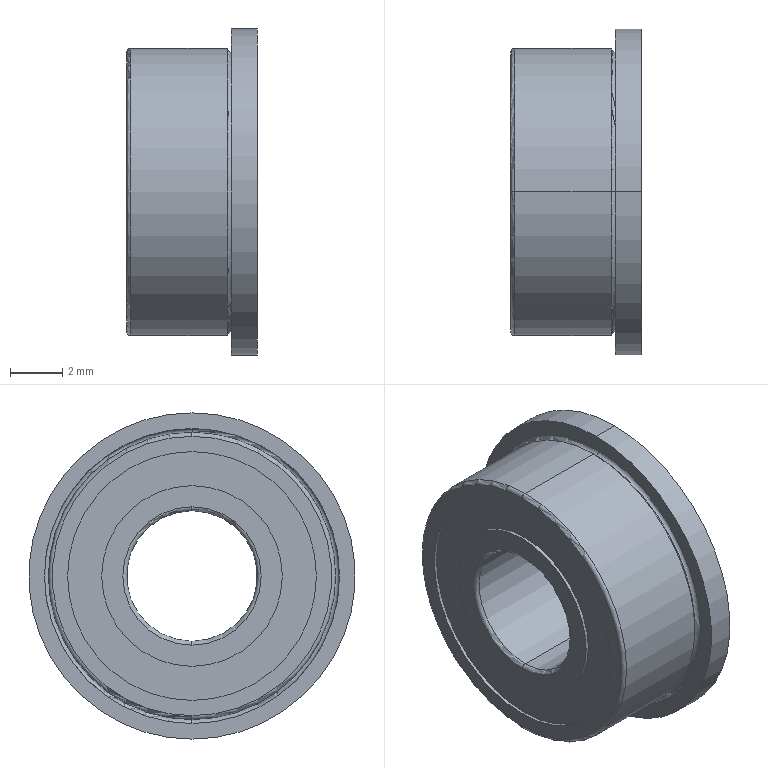Part | SolidWorks | features RefAxis 3, 3DProfileFeature 1, Revolution 1 | 1 solid | 31 faces | box 5 x 12.5 x 12.5 mm | volume 394.425 mm3 | cylinder 14 | torus 10 | plane 7 | commonest cylinder face diameters 6.92 x4 9.534 x4 5 x2 11 x2 12.5 x2
STEP:
#1=CARTESIAN_POINT('',(3.85,0.,5.5));
#2=VERTEX_POINT('',#1);
#3=CARTESIAN_POINT('',(4.,0.,5.35));
#4=VERTEX_POINT('',#3);
#5=CARTESIAN_POINT('',(4.,0.,5.5));
#6=DIRECTION('',(0.,-1.,0.));
#7=DIRECTION('',(0.,0.,-1.));
#8=AXIS2_PLACEMENT_3D('',#5,#6,#7);
#9=CIRCLE('',#8,0.15);
#10=EDGE_CURVE('',#2,#4,#9,.T.);
#11=ORIENTED_EDGE('',*,*,#10,.T.);
#12=CARTESIAN_POINT('',(4.,0.,-5.35));
#13=VERTEX_POINT('',#12);
#14=CARTESIAN_POINT('',(4.,0.,0.));
#15=DIRECTION('',(-1.,0.,0.));
#16=DIRECTION('',(0.,0.,1.));
#17=AXIS2_PLACEMENT_3D('',#14,#15,#16);
#18=CIRCLE('',#17,5.35);
#19=EDGE_CURVE('',#4,#13,#18,.T.);
#20=ORIENTED_EDGE('',*,*,#19,.T.);
#21=CARTESIAN_POINT('',(3.85,0.,-5.5));
#22=VERTEX_POINT('',#21);
#23=CARTESIAN_POINT('',(4.,0.,-5.5));
#24=DIRECTION('',(0.,1.,0.));
#25=DIRECTION('',(0.,0.,1.));
#26=AXIS2_PLACEMENT_3D('',#23,#24,#25);
#27=CIRCLE('',#26,0.15);
#28=EDGE_CURVE('',#22,#13,#27,.T.);
#29=ORIENTED_EDGE('',*,*,#28,.F.);
#30=CARTESIAN_POINT('',(3.85,0.,0.));
#31=DIRECTION('',(-1.,0.,0.));
#32=DIRECTION('',(0.,0.,1.));
#33=AXIS2_PLACEMENT_3D('',#30,#31,#32);
#34=CIRCLE('',#33,5.5);
#35=EDGE_CURVE('',#2,#22,#34,.T.);
#36=ORIENTED_EDGE('',*,*,#35,.F.);
#37=EDGE_LOOP('',(#11,#20,#29,#36));
#38=FACE_OUTER_BOUND('',#37,.T.);
#39=CARTESIAN_POINT('',(4.,0.,0.));
#40=DIRECTION('',(-1.,0.,0.));
#41=DIRECTION('',(0.,0.,1.));
#42=AXIS2_PLACEMENT_3D('',#39,#40,#41);
#43=TOROIDAL_SURFACE('',#42,5.5,0.15);
#44=ADVANCED_FACE('',(#38),#43,.F.);
#45=ORIENTED_EDGE('',*,*,#28,.T.);
#46=CARTESIAN_POINT('',(4.,0.,0.));
#47=DIRECTION('',(-1.,0.,0.));
#48=DIRECTION('',(0.,0.,1.));
#49=AXIS2_PLACEMENT_3D('',#46,#47,#48);
#50=CIRCLE('',#49,5.35);
#51=EDGE_CURVE('',#13,#4,#50,.T.);
#52=ORIENTED_EDGE('',*,*,#51,.T.);
#53=ORIENTED_EDGE('',*,*,#10,.F.);
#54=CARTESIAN_POINT('',(3.85,0.,0.));
#55=DIRECTION('',(-1.,0.,0.));
#56=DIRECTION('',(0.,0.,1.));
#57=AXIS2_PLACEMENT_3D('',#54,#55,#56);
#58=CIRCLE('',#57,5.5);
#59=EDGE_CURVE('',#22,#2,#58,.T.);
#60=ORIENTED_EDGE('',*,*,#59,.F.);
#61=EDGE_LOOP('',(#45,#52,#53,#60));
#62=FACE_OUTER_BOUND('',#61,.T.);
#63=CARTESIAN_POINT('',(4.,0.,0.));
#64=DIRECTION('',(-1.,0.,0.));
#65=DIRECTION('',(0.,0.,1.));
#66=AXIS2_PLACEMENT_3D('',#63,#64,#65);
#67=TOROIDAL_SURFACE('',#66,5.5,0.15);
#68=ADVANCED_FACE('',(#62),#67,.F.);
#69=ORIENTED_EDGE('',*,*,#35,.T.);
#70=CARTESIAN_POINT('',(0.15,0.,-5.5));
#71=VERTEX_POINT('',#70);
#72=CARTESIAN_POINT('',(11.,0.,-5.5));
#73=DIRECTION('',(-1.,0.,0.));
#74=VECTOR('',#73,1000.);
#75=LINE('',#72,#74);
#76=EDGE_CURVE('',#22,#71,#75,.T.);
#77=ORIENTED_EDGE('',*,*,#76,.T.);
#78=CARTESIAN_POINT('',(0.15,0.,5.5));
#79=VERTEX_POINT('',#78);
#80=CARTESIAN_POINT('',(0.15,0.,0.));
#81=DIRECTION('',(-1.,0.,0.));
#82=DIRECTION('',(0.,0.,1.));
#83=AXIS2_PLACEMENT_3D('',#80,#81,#82);
#84=CIRCLE('',#83,5.5);
#85=EDGE_CURVE('',#79,#71,#84,.T.);
#86=ORIENTED_EDGE('',*,*,#85,.F.);
#87=CARTESIAN_POINT('',(11.,0.,5.5));
#88=DIRECTION('',(-1.,0.,0.));
#89=VECTOR('',#88,1000.);
#90=LINE('',#87,#89);
#91=EDGE_CURVE('',#2,#79,#90,.T.);
#92=ORIENTED_EDGE('',*,*,#91,.F.);
#93=EDGE_LOOP('',(#69,#77,#86,#92));
#94=FACE_OUTER_BOUND('',#93,.T.);
#95=CARTESIAN_POINT('',(11.,0.,0.));
#96=DIRECTION('',(-1.,0.,0.));
#97=DIRECTION('',(0.,0.,1.));
#98=AXIS2_PLACEMENT_3D('',#95,#96,#97);
#99=CYLINDRICAL_SURFACE('',#98,5.5);
#100=ADVANCED_FACE('',(#94),#99,.T.);
#101=ORIENTED_EDGE('',*,*,#51,.F.);
#102=CARTESIAN_POINT('',(4.,0.,-5.65));
#103=VERTEX_POINT('',#102);
#104=CARTESIAN_POINT('',(4.,0.,-5.5));
#105=DIRECTION('',(0.,1.,0.));
#106=DIRECTION('',(0.,0.,1.));
#107=AXIS2_PLACEMENT_3D('',#104,#105,#106);
#108=CIRCLE('',#107,0.15);
#109=EDGE_CURVE('',#13,#103,#108,.T.);
#110=ORIENTED_EDGE('',*,*,#109,.T.);
#111=CARTESIAN_POINT('',(4.,0.,5.65));
#112=VERTEX_POINT('',#111);
#113=CARTESIAN_POINT('',(4.,0.,0.));
#114=DIRECTION('',(-1.,0.,0.));
#115=DIRECTION('',(0.,0.,1.));
#116=AXIS2_PLACEMENT_3D('',#113,#114,#115);
#117=CIRCLE('',#116,5.65);
#118=EDGE_CURVE('',#103,#112,#117,.T.);
#119=ORIENTED_EDGE('',*,*,#118,.T.);
#120=CARTESIAN_POINT('',(4.,0.,5.5));
#121=DIRECTION('',(0.,-1.,0.));
#122=DIRECTION('',(0.,0.,-1.));
#123=AXIS2_PLACEMENT_3D('',#120,#121,#122);
#124=CIRCLE('',#123,0.15);
#125=EDGE_CURVE('',#4,#112,#124,.T.);
#126=ORIENTED_EDGE('',*,*,#125,.F.);
#127=EDGE_LOOP('',(#101,#110,#119,#126));
#128=FACE_OUTER_BOUND('',#127,.T.);
#129=CARTESIAN_POINT('',(4.,0.,0.));
#130=DIRECTION('',(-1.,0.,0.));
#131=DIRECTION('',(0.,0.,1.));
#132=AXIS2_PLACEMENT_3D('',#129,#130,#131);
#133=TOROIDAL_SURFACE('',#132,5.5,0.15);
#134=ADVANCED_FACE('',(#128),#133,.F.);
#135=CARTESIAN_POINT('',(5.,0.,6.25));
#136=VERTEX_POINT('',#135);
#137=CARTESIAN_POINT('',(5.,0.,-6.25));
#138=VERTEX_POINT('',#137);
#139=CARTESIAN_POINT('',(5.,0.,0.));
#140=DIRECTION('',(-1.,0.,0.));
#141=DIRECTION('',(0.,0.,1.));
#142=AXIS2_PLACEMENT_3D('',#139,#140,#141);
#143=CIRCLE('',#142,6.25);
#144=EDGE_CURVE('',#136,#138,#143,.T.);
#145=ORIENTED_EDGE('',*,*,#144,.T.);
#146=CARTESIAN_POINT('',(4.,0.,-6.25));
#147=VERTEX_POINT('',#146);
#148=CARTESIAN_POINT('',(11.,0.,-6.25));
#149=DIRECTION('',(-1.,0.,0.));
#150=VECTOR('',#149,1000.);
#151=LINE('',#148,#150);
#152=EDGE_CURVE('',#138,#147,#151,.T.);
#153=ORIENTED_EDGE('',*,*,#152,.T.);
#154=CARTESIAN_POINT('',(4.,0.,6.25));
#155=VERTEX_POINT('',#154);
#156=CARTESIAN_POINT('',(4.,0.,0.));
#157=DIRECTION('',(-1.,0.,0.));
#158=DIRECTION('',(0.,0.,1.));
#159=AXIS2_PLACEMENT_3D('',#156,#157,#158);
#160=CIRCLE('',#159,6.25);
#161=EDGE_CURVE('',#155,#147,#160,.T.);
#162=ORIENTED_EDGE('',*,*,#161,.F.);
#163=CARTESIAN_POINT('',(11.,0.,6.25));
#164=DIRECTION('',(-1.,0.,0.));
#165=VECTOR('',#164,1000.);
#166=LINE('',#163,#165);
#167=EDGE_CURVE('',#136,#155,#166,.T.);
#168=ORIENTED_EDGE('',*,*,#167,.F.);
#169=EDGE_LOOP('',(#145,#153,#162,#168));
#170=FACE_OUTER_BOUND('',#169,.T.);
#171=CARTESIAN_POINT('',(11.,0.,0.));
#172=DIRECTION('',(-1.,0.,0.));
#173=DIRECTION('',(0.,0.,1.));
#174=AXIS2_PLACEMENT_3D('',#171,#172,#173);
#175=CYLINDRICAL_SURFACE('',#174,6.25);
#176=ADVANCED_FACE('',(#170),#175,.T.);
#177=CARTESIAN_POINT('',(5.,0.,-4.767));
#178=VERTEX_POINT('',#177);
#179=CARTESIAN_POINT('',(5.,0.,4.767));
#180=VERTEX_POINT('',#179);
#181=CARTESIAN_POINT('',(5.,0.,0.));
#182=DIRECTION('',(-1.,0.,0.));
#183=DIRECTION('',(0.,0.,1.));
#184=AXIS2_PLACEMENT_3D('',#181,#182,#183);
#185=CIRCLE('',#184,4.767);
#186=EDGE_CURVE('',#178,#180,#185,.T.);
#187=ORIENTED_EDGE('',*,*,#186,.F.);
#188=CARTESIAN_POINT('',(4.88,0.,-4.767));
#189=VERTEX_POINT('',#188);
#190=CARTESIAN_POINT('',(11.,0.,-4.767));
#191=DIRECTION('',(-1.,0.,0.));
#192=VECTOR('',#191,1000.);
#193=LINE('',#190,#192);
#194=EDGE_CURVE('',#178,#189,#193,.T.);
#195=ORIENTED_EDGE('',*,*,#194,.T.);
#196=CARTESIAN_POINT('',(4.88,0.,4.767));
#197=VERTEX_POINT('',#196);
#198=CARTESIAN_POINT('',(4.88,0.,0.));
#199=DIRECTION('',(-1.,0.,0.));
#200=DIRECTION('',(0.,0.,1.));
#201=AXIS2_PLACEMENT_3D('',#198,#199,#200);
#202=CIRCLE('',#201,4.767);
#203=EDGE_CURVE('',#189,#197,#202,.T.);
#204=ORIENTED_EDGE('',*,*,#203,.T.);
#205=CARTESIAN_POINT('',(11.,0.,4.767));
#206=DIRECTION('',(-1.,0.,0.));
#207=VECTOR('',#206,1000.);
#208=LINE('',#205,#207);
#209=EDGE_CURVE('',#180,#197,#208,.T.);
#210=ORIENTED_EDGE('',*,*,#209,.F.);
#211=EDGE_LOOP('',(#187,#195,#204,#210));
#212=FACE_OUTER_BOUND('',#211,.T.);
#213=CARTESIAN_POINT('',(11.,0.,0.));
#214=DIRECTION('',(-1.,0.,0.));
#215=DIRECTION('',(0.,0.,1.));
#216=AXIS2_PLACEMENT_3D('',#213,#214,#215);
#217=CYLINDRICAL_SURFACE('',#216,4.767);
#218=ADVANCED_FACE('',(#212),#217,.F.);
#219=CARTESIAN_POINT('',(5.,0.,3.46));
#220=VERTEX_POINT('',#219);
#221=CARTESIAN_POINT('',(5.,0.,-3.46));
#222=VERTEX_POINT('',#221);
#223=CARTESIAN_POINT('',(5.,0.,0.));
#224=DIRECTION('',(-1.,0.,0.));
#225=DIRECTION('',(0.,0.,1.));
#226=AXIS2_PLACEMENT_3D('',#223,#224,#225);
#227=CIRCLE('',#226,3.46);
#228=EDGE_CURVE('',#220,#222,#227,.T.);
#229=ORIENTED_EDGE('',*,*,#228,.T.);
#230=CARTESIAN_POINT('',(4.88,0.,-3.46));
#231=VERTEX_POINT('',#230);
#232=CARTESIAN_POINT('',(11.,0.,-3.46));
#233=DIRECTION('',(-1.,0.,0.));
#234=VECTOR('',#233,1000.);
#235=LINE('',#232,#234);
#236=EDGE_CURVE('',#222,#231,#235,.T.);
#237=ORIENTED_EDGE('',*,*,#236,.T.);
#238=CARTESIAN_POINT('',(4.88,0.,3.46));
#239=VERTEX_POINT('',#238);
#240=CARTESIAN_POINT('',(4.88,0.,0.));
#241=DIRECTION('',(-1.,0.,0.));
#242=DIRECTION('',(0.,0.,1.));
#243=AXIS2_PLACEMENT_3D('',#240,#241,#242);
#244=CIRCLE('',#243,3.46);
#245=EDGE_CURVE('',#239,#231,#244,.T.);
#246=ORIENTED_EDGE('',*,*,#245,.F.);
#247=CARTESIAN_POINT('',(11.,0.,3.46));
#248=DIRECTION('',(-1.,0.,0.));
#249=VECTOR('',#248,1000.);
#250=LINE('',#247,#249);
#251=EDGE_CURVE('',#220,#239,#250,.T.);
#252=ORIENTED_EDGE('',*,*,#251,.F.);
#253=EDGE_LOOP('',(#229,#237,#246,#252));
#254=FACE_OUTER_BOUND('',#253,.T.);
#255=CARTESIAN_POINT('',(11.,0.,0.));
#256=DIRECTION('',(-1.,0.,0.));
#257=DIRECTION('',(0.,0.,1.));
#258=AXIS2_PLACEMENT_3D('',#255,#256,#257);
#259=CYLINDRICAL_SURFACE('',#258,3.46);
#260=ADVANCED_FACE('',(#254),#259,.T.);
#261=CARTESIAN_POINT('',(4.85,0.,2.5));
#262=VERTEX_POINT('',#261);
#263=CARTESIAN_POINT('',(4.85,0.,-2.5));
#264=VERTEX_POINT('',#263);
#265=CARTESIAN_POINT('',(4.85,0.,0.));
#266=DIRECTION('',(-1.,0.,0.));
#267=DIRECTION('',(0.,0.,1.));
#268=AXIS2_PLACEMENT_3D('',#265,#266,#267);
#269=CIRCLE('',#268,2.5);
#270=EDGE_CURVE('',#262,#264,#269,.T.);
#271=ORIENTED_EDGE('',*,*,#270,.T.);
#272=CARTESIAN_POINT('',(5.,0.,-2.65));
#273=VERTEX_POINT('',#272);
#274=CARTESIAN_POINT('',(4.85,0.,-2.65));
#275=DIRECTION('',(0.,1.,0.));
#276=DIRECTION('',(0.,0.,1.));
#277=AXIS2_PLACEMENT_3D('',#274,#275,#276);
#278=CIRCLE('',#277,0.15);
#279=EDGE_CURVE('',#264,#273,#278,.T.);
#280=ORIENTED_EDGE('',*,*,#279,.T.);
#281=CARTESIAN_POINT('',(5.,0.,2.65));
#282=VERTEX_POINT('',#281);
#283=CARTESIAN_POINT('',(5.,0.,0.));
#284=DIRECTION('',(-1.,0.,0.));
#285=DIRECTION('',(0.,0.,1.));
#286=AXIS2_PLACEMENT_3D('',#283,#284,#285);
#287=CIRCLE('',#286,2.65);
#288=EDGE_CURVE('',#282,#273,#287,.T.);
#289=ORIENTED_EDGE('',*,*,#288,.F.);
#290=CARTESIAN_POINT('',(4.85,0.,2.65));
#291=DIRECTION('',(0.,-1.,0.));
#292=DIRECTION('',(0.,0.,-1.));
#293=AXIS2_PLACEMENT_3D('',#290,#291,#292);
#294=CIRCLE('',#293,0.15);
#295=EDGE_CURVE('',#262,#282,#294,.T.);
#296=ORIENTED_EDGE('',*,*,#295,.F.);
#297=EDGE_LOOP('',(#271,#280,#289,#296));
#298=FACE_OUTER_BOUND('',#297,.T.);
#299=CARTESIAN_POINT('',(4.85,0.,0.));
#300=DIRECTION('',(-1.,0.,0.));
#301=DIRECTION('',(0.,0.,1.));
#302=AXIS2_PLACEMENT_3D('',#299,#300,#301);
#303=TOROIDAL_SURFACE('',#302,2.65,0.15);
#304=ADVANCED_FACE('',(#298),#303,.T.);
#305=CARTESIAN_POINT('',(4.85,0.,0.));
#306=DIRECTION('',(-1.,0.,0.));
#307=DIRECTION('',(0.,0.,1.));
#308=AXIS2_PLACEMENT_3D('',#305,#306,#307);
#309=CIRCLE('',#308,2.5);
#310=EDGE_CURVE('',#264,#262,#309,.T.);
#311=ORIENTED_EDGE('',*,*,#310,.F.);
#312=CARTESIAN_POINT('',(0.15,0.,-2.5));
#313=VERTEX_POINT('',#312);
#314=CARTESIAN_POINT('',(11.,0.,-2.5));
#315=DIRECTION('',(-1.,0.,0.));
#316=VECTOR('',#315,1000.);
#317=LINE('',#314,#316);
#318=EDGE_CURVE('',#264,#313,#317,.T.);
#319=ORIENTED_EDGE('',*,*,#318,.T.);
#320=CARTESIAN_POINT('',(0.15,0.,2.5));
#321=VERTEX_POINT('',#320);
#322=CARTESIAN_POINT('',(0.15,0.,0.));
#323=DIRECTION('',(-1.,0.,0.));
#324=DIRECTION('',(0.,0.,1.));
#325=AXIS2_PLACEMENT_3D('',#322,#323,#324);
#326=CIRCLE('',#325,2.5);
#327=EDGE_CURVE('',#313,#321,#326,.T.);
#328=ORIENTED_EDGE('',*,*,#327,.T.);
#329=CARTESIAN_POINT('',(11.,0.,2.5));
#330=DIRECTION('',(-1.,0.,0.));
#331=VECTOR('',#330,1000.);
#332=LINE('',#329,#331);
#333=EDGE_CURVE('',#262,#321,#332,.T.);
#334=ORIENTED_EDGE('',*,*,#333,.F.);
#335=EDGE_LOOP('',(#311,#319,#328,#334));
#336=FACE_OUTER_BOUND('',#335,.T.);
#337=CARTESIAN_POINT('',(11.,0.,0.));
#338=DIRECTION('',(-1.,0.,0.));
#339=DIRECTION('',(0.,0.,1.));
#340=AXIS2_PLACEMENT_3D('',#337,#338,#339);
#341=CYLINDRICAL_SURFACE('',#340,2.5);
#342=ADVANCED_FACE('',(#336),#341,.F.);
#343=CARTESIAN_POINT('',(0.,0.,2.65));
#344=VERTEX_POINT('',#343);
#345=CARTESIAN_POINT('',(0.,0.,-2.65));
#346=VERTEX_POINT('',#345);
#347=CARTESIAN_POINT('',(0.,0.,0.));
#348=DIRECTION('',(-1.,0.,0.));
#349=DIRECTION('',(0.,0.,1.));
#350=AXIS2_PLACEMENT_3D('',#347,#348,#349);
#351=CIRCLE('',#350,2.65);
#352=EDGE_CURVE('',#344,#346,#351,.T.);
#353=ORIENTED_EDGE('',*,*,#352,.T.);
#354=CARTESIAN_POINT('',(0.15,0.,-2.65));
#355=DIRECTION('',(0.,1.,0.));
#356=DIRECTION('',(0.,0.,1.));
#357=AXIS2_PLACEMENT_3D('',#354,#355,#356);
#358=CIRCLE('',#357,0.15);
#359=EDGE_CURVE('',#346,#313,#358,.T.);
#360=ORIENTED_EDGE('',*,*,#359,.T.);
#361=CARTESIAN_POINT('',(0.15,0.,0.));
#362=DIRECTION('',(-1.,0.,0.));
#363=DIRECTION('',(0.,0.,1.));
#364=AXIS2_PLACEMENT_3D('',#361,#362,#363);
#365=CIRCLE('',#364,2.5);
#366=EDGE_CURVE('',#321,#313,#365,.T.);
#367=ORIENTED_EDGE('',*,*,#366,.F.);
#368=CARTESIAN_POINT('',(0.15,0.,2.65));
#369=DIRECTION('',(0.,-1.,0.));
#370=DIRECTION('',(0.,0.,-1.));
#371=AXIS2_PLACEMENT_3D('',#368,#369,#370);
#372=CIRCLE('',#371,0.15);
#373=EDGE_CURVE('',#344,#321,#372,.T.);
#374=ORIENTED_EDGE('',*,*,#373,.F.);
#375=EDGE_LOOP('',(#353,#360,#367,#374));
#376=FACE_OUTER_BOUND('',#375,.T.);
#377=CARTESIAN_POINT('',(0.15,0.,0.));
#378=DIRECTION('',(-1.,0.,0.));
#379=DIRECTION('',(0.,0.,1.));
#380=AXIS2_PLACEMENT_3D('',#377,#378,#379);
#381=TOROIDAL_SURFACE('',#380,2.65,0.15);
#382=ADVANCED_FACE('',(#376),#381,.T.);
#383=CARTESIAN_POINT('',(0.12,0.,3.46));
#384=VERTEX_POINT('',#383);
#385=CARTESIAN_POINT('',(0.12,0.,-3.46));
#386=VERTEX_POINT('',#385);
#387=CARTESIAN_POINT('',(0.12,0.,0.));
#388=DIRECTION('',(-1.,0.,0.));
#389=DIRECTION('',(0.,0.,1.));
#390=AXIS2_PLACEMENT_3D('',#387,#388,#389);
#391=CIRCLE('',#390,3.46);
#392=EDGE_CURVE('',#384,#386,#391,.T.);
#393=ORIENTED_EDGE('',*,*,#392,.T.);
#394=CARTESIAN_POINT('',(0.,0.,-3.46));
#395=VERTEX_POINT('',#394);
#396=CARTESIAN_POINT('',(11.,0.,-3.46));
#397=DIRECTION('',(-1.,0.,0.));
#398=VECTOR('',#397,1000.);
#399=LINE('',#396,#398);
#400=EDGE_CURVE('',#386,#395,#399,.T.);
#401=ORIENTED_EDGE('',*,*,#400,.T.);
#402=CARTESIAN_POINT('',(0.,0.,3.46));
#403=VERTEX_POINT('',#402);
#404=CARTESIAN_POINT('',(0.,0.,0.));
#405=DIRECTION('',(-1.,0.,0.));
#406=DIRECTION('',(0.,0.,1.));
#407=AXIS2_PLACEMENT_3D('',#404,#405,#406);
#408=CIRCLE('',#407,3.46);
#409=EDGE_CURVE('',#403,#395,#408,.T.);
#410=ORIENTED_EDGE('',*,*,#409,.F.);
#411=CARTESIAN_POINT('',(11.,0.,3.46));
#412=DIRECTION('',(-1.,0.,0.));
#413=VECTOR('',#412,1000.);
#414=LINE('',#411,#413);
#415=EDGE_CURVE('',#384,#403,#414,.T.);
#416=ORIENTED_EDGE('',*,*,#415,.F.);
#417=EDGE_LOOP('',(#393,#401,#410,#416));
#418=FACE_OUTER_BOUND('',#417,.T.);
#419=CARTESIAN_POINT('',(11.,0.,0.));
#420=DIRECTION('',(-1.,0.,0.));
#421=DIRECTION('',(0.,0.,1.));
#422=AXIS2_PLACEMENT_3D('',#419,#420,#421);
#423=CYLINDRICAL_SURFACE('',#422,3.46);
#424=ADVANCED_FACE('',(#418),#423,.T.);
#425=CARTESIAN_POINT('',(0.12,0.,-4.767));
#426=VERTEX_POINT('',#425);
#427=CARTESIAN_POINT('',(0.12,0.,4.767));
#428=VERTEX_POINT('',#427);
#429=CARTESIAN_POINT('',(0.12,0.,0.));
#430=DIRECTION('',(-1.,0.,0.));
#431=DIRECTION('',(0.,0.,1.));
#432=AXIS2_PLACEMENT_3D('',#429,#430,#431);
#433=CIRCLE('',#432,4.767);
#434=EDGE_CURVE('',#426,#428,#433,.T.);
#435=ORIENTED_EDGE('',*,*,#434,.F.);
#436=CARTESIAN_POINT('',(0.,0.,-4.767));
#437=VERTEX_POINT('',#436);
#438=CARTESIAN_POINT('',(11.,0.,-4.767));
#439=DIRECTION('',(-1.,0.,0.));
#440=VECTOR('',#439,1000.);
#441=LINE('',#438,#440);
#442=EDGE_CURVE('',#426,#437,#441,.T.);
#443=ORIENTED_EDGE('',*,*,#442,.T.);
#444=CARTESIAN_POINT('',(0.,0.,4.767));
#445=VERTEX_POINT('',#444);
#446=CARTESIAN_POINT('',(0.,0.,0.));
#447=DIRECTION('',(-1.,0.,0.));
#448=DIRECTION('',(0.,0.,1.));
#449=AXIS2_PLACEMENT_3D('',#446,#447,#448);
#450=CIRCLE('',#449,4.767);
#451=EDGE_CURVE('',#437,#445,#450,.T.);
#452=ORIENTED_EDGE('',*,*,#451,.T.);
#453=CARTESIAN_POINT('',(11.,0.,4.767));
#454=DIRECTION('',(-1.,0.,0.));
#455=VECTOR('',#454,1000.);
#456=LINE('',#453,#455);
#457=EDGE_CURVE('',#428,#445,#456,.T.);
#458=ORIENTED_EDGE('',*,*,#457,.F.);
#459=EDGE_LOOP('',(#435,#443,#452,#458));
#460=FACE_OUTER_BOUND('',#459,.T.);
#461=CARTESIAN_POINT('',(11.,0.,0.));
#462=DIRECTION('',(-1.,0.,0.));
#463=DIRECTION('',(0.,0.,1.));
#464=AXIS2_PLACEMENT_3D('',#461,#462,#463);
#465=CYLINDRICAL_SURFACE('',#464,4.767);
#466=ADVANCED_FACE('',(#460),#465,.F.);
#467=ORIENTED_EDGE('',*,*,#85,.T.);
#468=CARTESIAN_POINT('',(0.,0.,-5.35));
#469=VERTEX_POINT('',#468);
#470=CARTESIAN_POINT('',(0.15,0.,-5.35));
#471=DIRECTION('',(0.,1.,0.));
#472=DIRECTION('',(0.,0.,1.));
#473=AXIS2_PLACEMENT_3D('',#470,#471,#472);
#474=CIRCLE('',#473,0.15);
#475=EDGE_CURVE('',#71,#469,#474,.T.);
#476=ORIENTED_EDGE('',*,*,#475,.T.);
#477=CARTESIAN_POINT('',(0.,0.,5.35));
#478=VERTEX_POINT('',#477);
#479=CARTESIAN_POINT('',(0.,0.,0.));
#480=DIRECTION('',(-1.,0.,0.));
#481=DIRECTION('',(0.,0.,1.));
#482=AXIS2_PLACEMENT_3D('',#479,#480,#481);
#483=CIRCLE('',#482,5.35);
#484=EDGE_CURVE('',#478,#469,#483,.T.);
#485=ORIENTED_EDGE('',*,*,#484,.F.);
#486=CARTESIAN_POINT('',(0.15,0.,5.35));
#487=DIRECTION('',(0.,-1.,0.));
#488=DIRECTION('',(0.,0.,-1.));
#489=AXIS2_PLACEMENT_3D('',#486,#487,#488);
#490=CIRCLE('',#489,0.15);
#491=EDGE_CURVE('',#79,#478,#490,.T.);
#492=ORIENTED_EDGE('',*,*,#491,.F.);
#493=EDGE_LOOP('',(#467,#476,#485,#492));
#494=FACE_OUTER_BOUND('',#493,.T.);
#495=CARTESIAN_POINT('',(0.15,0.,0.));
#496=DIRECTION('',(-1.,0.,0.));
#497=DIRECTION('',(0.,0.,1.));
#498=AXIS2_PLACEMENT_3D('',#495,#496,#497);
#499=TOROIDAL_SURFACE('',#498,5.35,0.15);
#500=ADVANCED_FACE('',(#494),#499,.T.);
#501=ORIENTED_EDGE('',*,*,#475,.F.);
#502=CARTESIAN_POINT('',(0.15,0.,0.));
#503=DIRECTION('',(-1.,0.,0.));
#504=DIRECTION('',(0.,0.,1.));
#505=AXIS2_PLACEMENT_3D('',#502,#503,#504);
#506=CIRCLE('',#505,5.5);
#507=EDGE_CURVE('',#71,#79,#506,.T.);
#508=ORIENTED_EDGE('',*,*,#507,.T.);
#509=ORIENTED_EDGE('',*,*,#491,.T.);
#510=CARTESIAN_POINT('',(0.,0.,0.));
#511=DIRECTION('',(-1.,0.,0.));
#512=DIRECTION('',(0.,0.,1.));
#513=AXIS2_PLACEMENT_3D('',#510,#511,#512);
#514=CIRCLE('',#513,5.35);
#515=EDGE_CURVE('',#469,#478,#514,.T.);
#516=ORIENTED_EDGE('',*,*,#515,.F.);
#517=EDGE_LOOP('',(#501,#508,#509,#516));
#518=FACE_OUTER_BOUND('',#517,.T.);
#519=CARTESIAN_POINT('',(0.15,0.,0.));
#520=DIRECTION('',(-1.,0.,0.));
#521=DIRECTION('',(0.,0.,1.));
#522=AXIS2_PLACEMENT_3D('',#519,#520,#521);
#523=TOROIDAL_SURFACE('',#522,5.35,0.15);
#524=ADVANCED_FACE('',(#518),#523,.T.);
#525=CARTESIAN_POINT('',(0.,0.,0.));
#526=DIRECTION('',(-1.,0.,0.));
#527=DIRECTION('',(0.,0.,1.));
#528=AXIS2_PLACEMENT_3D('',#525,#526,#527);
#529=CIRCLE('',#528,4.767);
#530=EDGE_CURVE('',#445,#437,#529,.T.);
#531=ORIENTED_EDGE('',*,*,#530,.F.);
#532=ORIENTED_EDGE('',*,*,#451,.F.);
#533=EDGE_LOOP('',(#531,#532));
#534=FACE_BOUND('',#533,.T.);
#535=ORIENTED_EDGE('',*,*,#484,.T.);
#536=ORIENTED_EDGE('',*,*,#515,.T.);
#537=EDGE_LOOP('',(#535,#536));
#538=FACE_OUTER_BOUND('',#537,.T.);
#539=CARTESIAN_POINT('',(0.,5.35,0.));
#540=DIRECTION('',(1.,0.,0.));
#541=DIRECTION('',(0.,0.,-1.));
#542=AXIS2_PLACEMENT_3D('',#539,#540,#541);
#543=PLANE('',#542);
#544=ADVANCED_FACE('',(#534,#538),#543,.F.);
#545=ORIENTED_EDGE('',*,*,#442,.F.);
#546=CARTESIAN_POINT('',(0.12,0.,0.));
#547=DIRECTION('',(-1.,0.,0.));
#548=DIRECTION('',(0.,0.,1.));
#549=AXIS2_PLACEMENT_3D('',#546,#547,#548);
#550=CIRCLE('',#549,4.767);
#551=EDGE_CURVE('',#428,#426,#550,.T.);
#552=ORIENTED_EDGE('',*,*,#551,.F.);
#553=ORIENTED_EDGE('',*,*,#457,.T.);
#554=ORIENTED_EDGE('',*,*,#530,.T.);
#555=EDGE_LOOP('',(#545,#552,#553,#554));
#556=FACE_OUTER_BOUND('',#555,.T.);
#557=CARTESIAN_POINT('',(11.,0.,0.));
#558=DIRECTION('',(-1.,0.,0.));
#559=DIRECTION('',(0.,0.,1.));
#560=AXIS2_PLACEMENT_3D('',#557,#558,#559);
#561=CYLINDRICAL_SURFACE('',#560,4.767);
#562=ADVANCED_FACE('',(#556),#561,.F.);
#563=ORIENTED_EDGE('',*,*,#392,.F.);
#564=CARTESIAN_POINT('',(0.12,0.,0.));
#565=DIRECTION('',(-1.,0.,0.));
#566=DIRECTION('',(0.,0.,1.));
#567=AXIS2_PLACEMENT_3D('',#564,#565,#566);
#568=CIRCLE('',#567,3.46);
#569=EDGE_CURVE('',#386,#384,#568,.T.);
#570=ORIENTED_EDGE('',*,*,#569,.F.);
#571=EDGE_LOOP('',(#563,#570));
#572=FACE_BOUND('',#571,.T.);
#573=ORIENTED_EDGE('',*,*,#551,.T.);
#574=ORIENTED_EDGE('',*,*,#434,.T.);
#575=EDGE_LOOP('',(#573,#574));
#576=FACE_OUTER_BOUND('',#575,.T.);
#577=CARTESIAN_POINT('',(0.12,4.767,0.));
#578=DIRECTION('',(1.,0.,0.));
#579=DIRECTION('',(0.,0.,-1.));
#580=AXIS2_PLACEMENT_3D('',#577,#578,#579);
#581=PLANE('',#580);
#582=ADVANCED_FACE('',(#572,#576),#581,.F.);
#583=ORIENTED_EDGE('',*,*,#400,.F.);
#584=ORIENTED_EDGE('',*,*,#569,.T.);
#585=ORIENTED_EDGE('',*,*,#415,.T.);
#586=CARTESIAN_POINT('',(0.,0.,0.));
#587=DIRECTION('',(-1.,0.,0.));
#588=DIRECTION('',(0.,0.,1.));
#589=AXIS2_PLACEMENT_3D('',#586,#587,#588);
#590=CIRCLE('',#589,3.46);
#591=EDGE_CURVE('',#395,#403,#590,.T.);
#592=ORIENTED_EDGE('',*,*,#591,.F.);
#593=EDGE_LOOP('',(#583,#584,#585,#592));
#594=FACE_OUTER_BOUND('',#593,.T.);
#595=CARTESIAN_POINT('',(11.,0.,0.));
#596=DIRECTION('',(-1.,0.,0.));
#597=DIRECTION('',(0.,0.,1.));
#598=AXIS2_PLACEMENT_3D('',#595,#596,#597);
#599=CYLINDRICAL_SURFACE('',#598,3.46);
#600=ADVANCED_FACE('',(#594),#599,.T.);
#601=ORIENTED_EDGE('',*,*,#352,.F.);
#602=CARTESIAN_POINT('',(0.,0.,0.));
#603=DIRECTION('',(-1.,0.,0.));
#604=DIRECTION('',(0.,0.,1.));
#605=AXIS2_PLACEMENT_3D('',#602,#603,#604);
#606=CIRCLE('',#605,2.65);
#607=EDGE_CURVE('',#346,#344,#606,.T.);
#608=ORIENTED_EDGE('',*,*,#607,.F.);
#609=EDGE_LOOP('',(#601,#608));
#610=FACE_BOUND('',#609,.T.);
#611=ORIENTED_EDGE('',*,*,#409,.T.);
#612=ORIENTED_EDGE('',*,*,#591,.T.);
#613=EDGE_LOOP('',(#611,#612));
#614=FACE_OUTER_BOUND('',#613,.T.);
#615=CARTESIAN_POINT('',(0.,3.46,0.));
#616=DIRECTION('',(1.,0.,0.));
#617=DIRECTION('',(0.,0.,-1.));
#618=AXIS2_PLACEMENT_3D('',#615,#616,#617);
#619=PLANE('',#618);
#620=ADVANCED_FACE('',(#610,#614),#619,.F.);
#621=ORIENTED_EDGE('',*,*,#359,.F.);
#622=ORIENTED_EDGE('',*,*,#607,.T.);
#623=ORIENTED_EDGE('',*,*,#373,.T.);
#624=ORIENTED_EDGE('',*,*,#327,.F.);
#625=EDGE_LOOP('',(#621,#622,#623,#624));
#626=FACE_OUTER_BOUND('',#625,.T.);
#627=CARTESIAN_POINT('',(0.15,0.,0.));
#628=DIRECTION('',(-1.,0.,0.));
#629=DIRECTION('',(0.,0.,1.));
#630=AXIS2_PLACEMENT_3D('',#627,#628,#629);
#631=TOROIDAL_SURFACE('',#630,2.65,0.15);
#632=ADVANCED_FACE('',(#626),#631,.T.);
#633=ORIENTED_EDGE('',*,*,#318,.F.);
#634=ORIENTED_EDGE('',*,*,#270,.F.);
#635=ORIENTED_EDGE('',*,*,#333,.T.);
#636=ORIENTED_EDGE('',*,*,#366,.T.);
#637=EDGE_LOOP('',(#633,#634,#635,#636));
#638=FACE_OUTER_BOUND('',#637,.T.);
#639=CARTESIAN_POINT('',(11.,0.,0.));
#640=DIRECTION('',(-1.,0.,0.));
#641=DIRECTION('',(0.,0.,1.));
#642=AXIS2_PLACEMENT_3D('',#639,#640,#641);
#643=CYLINDRICAL_SURFACE('',#642,2.5);
#644=ADVANCED_FACE('',(#638),#643,.F.);
#645=ORIENTED_EDGE('',*,*,#279,.F.);
#646=ORIENTED_EDGE('',*,*,#310,.T.);
#647=ORIENTED_EDGE('',*,*,#295,.T.);
#648=CARTESIAN_POINT('',(5.,0.,0.));
#649=DIRECTION('',(-1.,0.,0.));
#650=DIRECTION('',(0.,0.,1.));
#651=AXIS2_PLACEMENT_3D('',#648,#649,#650);
#652=CIRCLE('',#651,2.65);
#653=EDGE_CURVE('',#273,#282,#652,.T.);
#654=ORIENTED_EDGE('',*,*,#653,.F.);
#655=EDGE_LOOP('',(#645,#646,#647,#654));
#656=FACE_OUTER_BOUND('',#655,.T.);
#657=CARTESIAN_POINT('',(4.85,0.,0.));
#658=DIRECTION('',(-1.,0.,0.));
#659=DIRECTION('',(0.,0.,1.));
#660=AXIS2_PLACEMENT_3D('',#657,#658,#659);
#661=TOROIDAL_SURFACE('',#660,2.65,0.15);
#662=ADVANCED_FACE('',(#656),#661,.T.);
#663=ORIENTED_EDGE('',*,*,#228,.F.);
#664=CARTESIAN_POINT('',(5.,0.,0.));
#665=DIRECTION('',(-1.,0.,0.));
#666=DIRECTION('',(0.,0.,1.));
#667=AXIS2_PLACEMENT_3D('',#664,#665,#666);
#668=CIRCLE('',#667,3.46);
#669=EDGE_CURVE('',#222,#220,#668,.T.);
#670=ORIENTED_EDGE('',*,*,#669,.F.);
#671=EDGE_LOOP('',(#663,#670));
#672=FACE_OUTER_BOUND('',#671,.T.);
#673=ORIENTED_EDGE('',*,*,#288,.T.);
#674=ORIENTED_EDGE('',*,*,#653,.T.);
#675=EDGE_LOOP('',(#673,#674));
#676=FACE_BOUND('',#675,.T.);
#677=CARTESIAN_POINT('',(5.,2.65,0.));
#678=DIRECTION('',(-1.,0.,0.));
#679=DIRECTION('',(0.,0.,1.));
#680=AXIS2_PLACEMENT_3D('',#677,#678,#679);
#681=PLANE('',#680);
#682=ADVANCED_FACE('',(#672,#676),#681,.F.);
#683=ORIENTED_EDGE('',*,*,#236,.F.);
#684=ORIENTED_EDGE('',*,*,#669,.T.);
#685=ORIENTED_EDGE('',*,*,#251,.T.);
#686=CARTESIAN_POINT('',(4.88,0.,0.));
#687=DIRECTION('',(-1.,0.,0.));
#688=DIRECTION('',(0.,0.,1.));
#689=AXIS2_PLACEMENT_3D('',#686,#687,#688);
#690=CIRCLE('',#689,3.46);
#691=EDGE_CURVE('',#231,#239,#690,.T.);
#692=ORIENTED_EDGE('',*,*,#691,.F.);
#693=EDGE_LOOP('',(#683,#684,#685,#692));
#694=FACE_OUTER_BOUND('',#693,.T.);
#695=CARTESIAN_POINT('',(11.,0.,0.));
#696=DIRECTION('',(-1.,0.,0.));
#697=DIRECTION('',(0.,0.,1.));
#698=AXIS2_PLACEMENT_3D('',#695,#696,#697);
#699=CYLINDRICAL_SURFACE('',#698,3.46);
#700=ADVANCED_FACE('',(#694),#699,.T.);
#701=CARTESIAN_POINT('',(4.88,0.,0.));
#702=DIRECTION('',(-1.,0.,0.));
#703=DIRECTION('',(0.,0.,1.));
#704=AXIS2_PLACEMENT_3D('',#701,#702,#703);
#705=CIRCLE('',#704,4.767);
#706=EDGE_CURVE('',#197,#189,#705,.T.);
#707=ORIENTED_EDGE('',*,*,#706,.F.);
#708=ORIENTED_EDGE('',*,*,#203,.F.);
#709=EDGE_LOOP('',(#707,#708));
#710=FACE_OUTER_BOUND('',#709,.T.);
#711=ORIENTED_EDGE('',*,*,#245,.T.);
#712=ORIENTED_EDGE('',*,*,#691,.T.);
#713=EDGE_LOOP('',(#711,#712));
#714=FACE_BOUND('',#713,.T.);
#715=CARTESIAN_POINT('',(4.88,3.46,0.));
#716=DIRECTION('',(-1.,0.,0.));
#717=DIRECTION('',(0.,0.,1.));
#718=AXIS2_PLACEMENT_3D('',#715,#716,#717);
#719=PLANE('',#718);
#720=ADVANCED_FACE('',(#710,#714),#719,.F.);
#721=ORIENTED_EDGE('',*,*,#194,.F.);
#722=CARTESIAN_POINT('',(5.,0.,0.));
#723=DIRECTION('',(-1.,0.,0.));
#724=DIRECTION('',(0.,0.,1.));
#725=AXIS2_PLACEMENT_3D('',#722,#723,#724);
#726=CIRCLE('',#725,4.767);
#727=EDGE_CURVE('',#180,#178,#726,.T.);
#728=ORIENTED_EDGE('',*,*,#727,.F.);
#729=ORIENTED_EDGE('',*,*,#209,.T.);
#730=ORIENTED_EDGE('',*,*,#706,.T.);
#731=EDGE_LOOP('',(#721,#728,#729,#730));
#732=FACE_OUTER_BOUND('',#731,.T.);
#733=CARTESIAN_POINT('',(11.,0.,0.));
#734=DIRECTION('',(-1.,0.,0.));
#735=DIRECTION('',(0.,0.,1.));
#736=AXIS2_PLACEMENT_3D('',#733,#734,#735);
#737=CYLINDRICAL_SURFACE('',#736,4.767);
#738=ADVANCED_FACE('',(#732),#737,.F.);
#739=ORIENTED_EDGE('',*,*,#144,.F.);
#740=CARTESIAN_POINT('',(5.,0.,0.));
#741=DIRECTION('',(-1.,0.,0.));
#742=DIRECTION('',(0.,0.,1.));
#743=AXIS2_PLACEMENT_3D('',#740,#741,#742);
#744=CIRCLE('',#743,6.25);
#745=EDGE_CURVE('',#138,#136,#744,.T.);
#746=ORIENTED_EDGE('',*,*,#745,.F.);
#747=EDGE_LOOP('',(#739,#746));
#748=FACE_OUTER_BOUND('',#747,.T.);
#749=ORIENTED_EDGE('',*,*,#727,.T.);
#750=ORIENTED_EDGE('',*,*,#186,.T.);
#751=EDGE_LOOP('',(#749,#750));
#752=FACE_BOUND('',#751,.T.);
#753=CARTESIAN_POINT('',(5.,4.767,0.));
#754=DIRECTION('',(-1.,0.,0.));
#755=DIRECTION('',(0.,0.,1.));
#756=AXIS2_PLACEMENT_3D('',#753,#754,#755);
#757=PLANE('',#756);
#758=ADVANCED_FACE('',(#748,#752),#757,.F.);
#759=ORIENTED_EDGE('',*,*,#152,.F.);
#760=ORIENTED_EDGE('',*,*,#745,.T.);
#761=ORIENTED_EDGE('',*,*,#167,.T.);
#762=CARTESIAN_POINT('',(4.,0.,0.));
#763=DIRECTION('',(-1.,0.,0.));
#764=DIRECTION('',(0.,0.,1.));
#765=AXIS2_PLACEMENT_3D('',#762,#763,#764);
#766=CIRCLE('',#765,6.25);
#767=EDGE_CURVE('',#147,#155,#766,.T.);
#768=ORIENTED_EDGE('',*,*,#767,.F.);
#769=EDGE_LOOP('',(#759,#760,#761,#768));
#770=FACE_OUTER_BOUND('',#769,.T.);
#771=CARTESIAN_POINT('',(11.,0.,0.));
#772=DIRECTION('',(-1.,0.,0.));
#773=DIRECTION('',(0.,0.,1.));
#774=AXIS2_PLACEMENT_3D('',#771,#772,#773);
#775=CYLINDRICAL_SURFACE('',#774,6.25);
#776=ADVANCED_FACE('',(#770),#775,.T.);
#777=CARTESIAN_POINT('',(4.,0.,0.));
#778=DIRECTION('',(-1.,0.,0.));
#779=DIRECTION('',(0.,0.,1.));
#780=AXIS2_PLACEMENT_3D('',#777,#778,#779);
#781=CIRCLE('',#780,5.65);
#782=EDGE_CURVE('',#112,#103,#781,.T.);
#783=ORIENTED_EDGE('',*,*,#782,.F.);
#784=ORIENTED_EDGE('',*,*,#118,.F.);
#785=EDGE_LOOP('',(#783,#784));
#786=FACE_BOUND('',#785,.T.);
#787=ORIENTED_EDGE('',*,*,#161,.T.);
#788=ORIENTED_EDGE('',*,*,#767,.T.);
#789=EDGE_LOOP('',(#787,#788));
#790=FACE_OUTER_BOUND('',#789,.T.);
#791=CARTESIAN_POINT('',(4.,6.25,0.));
#792=DIRECTION('',(1.,0.,0.));
#793=DIRECTION('',(0.,0.,-1.));
#794=AXIS2_PLACEMENT_3D('',#791,#792,#793);
#795=PLANE('',#794);
#796=ADVANCED_FACE('',(#786,#790),#795,.F.);
#797=ORIENTED_EDGE('',*,*,#19,.F.);
#798=ORIENTED_EDGE('',*,*,#125,.T.);
#799=ORIENTED_EDGE('',*,*,#782,.T.);
#800=ORIENTED_EDGE('',*,*,#109,.F.);
#801=EDGE_LOOP('',(#797,#798,#799,#800));
#802=FACE_OUTER_BOUND('',#801,.T.);
#803=CARTESIAN_POINT('',(4.,0.,0.));
#804=DIRECTION('',(-1.,0.,0.));
#805=DIRECTION('',(0.,0.,1.));
#806=AXIS2_PLACEMENT_3D('',#803,#804,#805);
#807=TOROIDAL_SURFACE('',#806,5.5,0.15);
#808=ADVANCED_FACE('',(#802),#807,.F.);
#809=ORIENTED_EDGE('',*,*,#76,.F.);
#810=ORIENTED_EDGE('',*,*,#59,.T.);
#811=ORIENTED_EDGE('',*,*,#91,.T.);
#812=ORIENTED_EDGE('',*,*,#507,.F.);
#813=EDGE_LOOP('',(#809,#810,#811,#812));
#814=FACE_OUTER_BOUND('',#813,.T.);
#815=CARTESIAN_POINT('',(11.,0.,0.));
#816=DIRECTION('',(-1.,0.,0.));
#817=DIRECTION('',(0.,0.,1.));
#818=AXIS2_PLACEMENT_3D('',#815,#816,#817);
#819=CYLINDRICAL_SURFACE('',#818,5.5);
#820=ADVANCED_FACE('',(#814),#819,.T.);
#821=CLOSED_SHELL('',(#44,#68,#100,#134,#176,#218,#260,#304,#342,#382,#424,#466,#500,#524,#544,#562,#582,#600,#620,#632,#644,#662,#682,#700,#720,#738,#758,#776,#796,#808,#820));
#822=MANIFOLD_SOLID_BREP('',#821);
#823=CARTESIAN_POINT('',(0.,0.,0.));
#824=DIRECTION('',(0.,0.,1.));
#825=DIRECTION('',(1.,0.,0.));
#826=AXIS2_PLACEMENT_3D('',#823,#824,#825);
#827=(LENGTH_UNIT()NAMED_UNIT(*)SI_UNIT(.MILLI.,.METRE.));
#828=UNCERTAINTY_MEASURE_WITH_UNIT(LENGTH_MEASURE(0.00001),#827,'','');
#829=(NAMED_UNIT(*)PLANE_ANGLE_UNIT()SI_UNIT($,.RADIAN.));
#830=(NAMED_UNIT(*)SI_UNIT($,.STERADIAN.)SOLID_ANGLE_UNIT());
#831=(GEOMETRIC_REPRESENTATION_CONTEXT(3)GLOBAL_UNCERTAINTY_ASSIGNED_CONTEXT((#828))GLOBAL_UNIT_ASSIGNED_CONTEXT((#827,#829,#830))REPRESENTATION_CONTEXT('',''));
#832=ADVANCED_BREP_SHAPE_REPRESENTATION('',(#822,#826),#831);